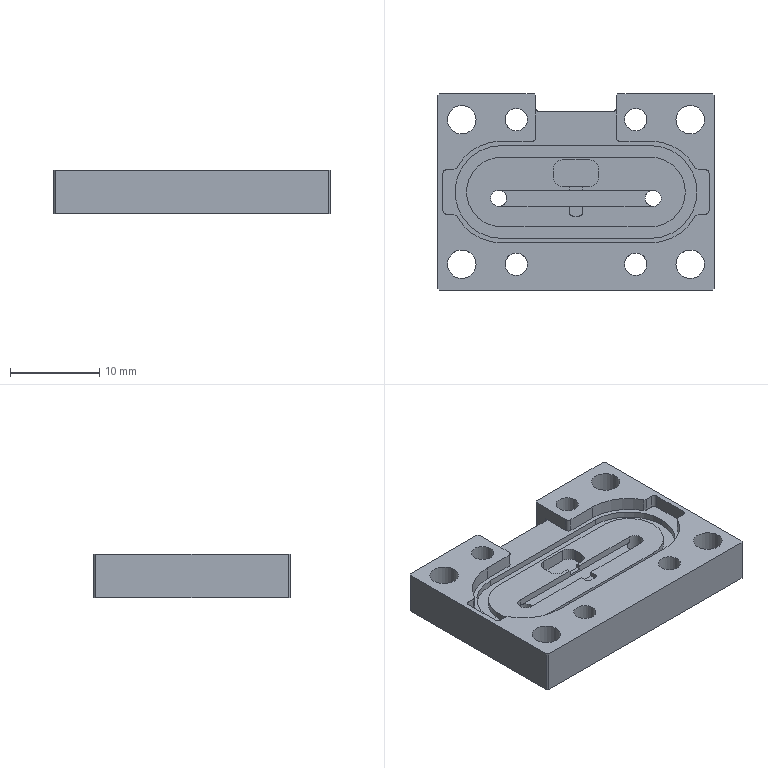Part | 1 solid | 89 faces | box 31 x 22 x 4.9 mm | volume 2385 mm3 | plane 53 | cylinder 36 | commonest cylinder face diameters 0.8 x10 10.4 x5 2 x4 2.5 x4 3.2 x4 11.4 x4